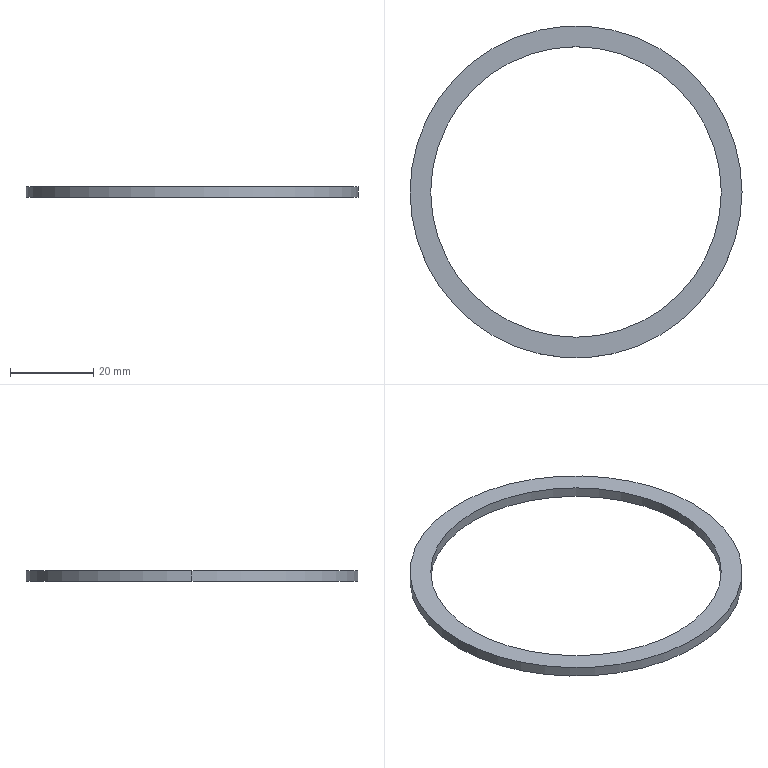Part | SolidWorks | features Extrusion 1 | 1 solid | 6 faces | box 80 x 80 x 2.5 mm | volume 2945 mm3 | cylinder 4 | plane 2 | commonest cylinder face diameters 70 x2 80 x2
STEP:
#1=CARTESIAN_POINT('',(-35.,0.,2.5));
#2=VERTEX_POINT('',#1);
#3=CARTESIAN_POINT('',(35.,0.,2.5));
#4=VERTEX_POINT('',#3);
#5=CARTESIAN_POINT('',(0.,0.,2.5));
#6=DIRECTION('',(0.,0.,1.));
#7=DIRECTION('',(1.,0.,0.));
#8=AXIS2_PLACEMENT_3D('',#5,#6,#7);
#9=CIRCLE('',#8,35.);
#10=EDGE_CURVE('',#2,#4,#9,.T.);
#11=ORIENTED_EDGE('',*,*,#10,.T.);
#12=CARTESIAN_POINT('',(35.,0.,0.));
#13=VERTEX_POINT('',#12);
#14=CARTESIAN_POINT('',(35.,0.,2.5));
#15=DIRECTION('',(0.,0.,-1.));
#16=VECTOR('',#15,1000.);
#17=LINE('',#14,#16);
#18=EDGE_CURVE('',#4,#13,#17,.T.);
#19=ORIENTED_EDGE('',*,*,#18,.T.);
#20=CARTESIAN_POINT('',(-35.,0.,0.));
#21=VERTEX_POINT('',#20);
#22=CARTESIAN_POINT('',(0.,0.,0.));
#23=DIRECTION('',(0.,0.,1.));
#24=DIRECTION('',(1.,0.,0.));
#25=AXIS2_PLACEMENT_3D('',#22,#23,#24);
#26=CIRCLE('',#25,35.);
#27=EDGE_CURVE('',#21,#13,#26,.T.);
#28=ORIENTED_EDGE('',*,*,#27,.F.);
#29=CARTESIAN_POINT('',(-35.,0.,2.5));
#30=DIRECTION('',(0.,0.,-1.));
#31=VECTOR('',#30,1000.);
#32=LINE('',#29,#31);
#33=EDGE_CURVE('',#2,#21,#32,.T.);
#34=ORIENTED_EDGE('',*,*,#33,.F.);
#35=EDGE_LOOP('',(#11,#19,#28,#34));
#36=FACE_OUTER_BOUND('',#35,.T.);
#37=CARTESIAN_POINT('',(0.,0.,2.5));
#38=DIRECTION('',(0.,0.,-1.));
#39=DIRECTION('',(-1.,0.,0.));
#40=AXIS2_PLACEMENT_3D('',#37,#38,#39);
#41=CYLINDRICAL_SURFACE('',#40,35.);
#42=ADVANCED_FACE('',(#36),#41,.F.);
#43=CARTESIAN_POINT('',(40.,0.,2.5));
#44=VERTEX_POINT('',#43);
#45=CARTESIAN_POINT('',(-40.,0.,2.5));
#46=VERTEX_POINT('',#45);
#47=CARTESIAN_POINT('',(0.,0.,2.5));
#48=DIRECTION('',(0.,0.,1.));
#49=DIRECTION('',(1.,0.,0.));
#50=AXIS2_PLACEMENT_3D('',#47,#48,#49);
#51=CIRCLE('',#50,40.);
#52=EDGE_CURVE('',#44,#46,#51,.T.);
#53=ORIENTED_EDGE('',*,*,#52,.F.);
#54=CARTESIAN_POINT('',(40.,0.,0.));
#55=VERTEX_POINT('',#54);
#56=CARTESIAN_POINT('',(40.,0.,2.5));
#57=DIRECTION('',(0.,0.,-1.));
#58=VECTOR('',#57,1000.);
#59=LINE('',#56,#58);
#60=EDGE_CURVE('',#44,#55,#59,.T.);
#61=ORIENTED_EDGE('',*,*,#60,.T.);
#62=CARTESIAN_POINT('',(-40.,0.,0.));
#63=VERTEX_POINT('',#62);
#64=CARTESIAN_POINT('',(0.,0.,0.));
#65=DIRECTION('',(0.,0.,1.));
#66=DIRECTION('',(1.,0.,0.));
#67=AXIS2_PLACEMENT_3D('',#64,#65,#66);
#68=CIRCLE('',#67,40.);
#69=EDGE_CURVE('',#55,#63,#68,.T.);
#70=ORIENTED_EDGE('',*,*,#69,.T.);
#71=CARTESIAN_POINT('',(-40.,0.,2.5));
#72=DIRECTION('',(0.,0.,-1.));
#73=VECTOR('',#72,1000.);
#74=LINE('',#71,#73);
#75=EDGE_CURVE('',#46,#63,#74,.T.);
#76=ORIENTED_EDGE('',*,*,#75,.F.);
#77=EDGE_LOOP('',(#53,#61,#70,#76));
#78=FACE_OUTER_BOUND('',#77,.T.);
#79=CARTESIAN_POINT('',(0.,0.,2.5));
#80=DIRECTION('',(0.,0.,-1.));
#81=DIRECTION('',(-1.,0.,0.));
#82=AXIS2_PLACEMENT_3D('',#79,#80,#81);
#83=CYLINDRICAL_SURFACE('',#82,40.);
#84=ADVANCED_FACE('',(#78),#83,.T.);
#85=CARTESIAN_POINT('',(0.,0.,2.5));
#86=DIRECTION('',(0.,0.,1.));
#87=DIRECTION('',(1.,0.,0.));
#88=AXIS2_PLACEMENT_3D('',#85,#86,#87);
#89=CIRCLE('',#88,40.);
#90=EDGE_CURVE('',#46,#44,#89,.T.);
#91=ORIENTED_EDGE('',*,*,#90,.T.);
#92=ORIENTED_EDGE('',*,*,#52,.T.);
#93=EDGE_LOOP('',(#91,#92));
#94=FACE_OUTER_BOUND('',#93,.T.);
#95=ORIENTED_EDGE('',*,*,#10,.F.);
#96=CARTESIAN_POINT('',(0.,0.,2.5));
#97=DIRECTION('',(0.,0.,1.));
#98=DIRECTION('',(1.,0.,0.));
#99=AXIS2_PLACEMENT_3D('',#96,#97,#98);
#100=CIRCLE('',#99,35.);
#101=EDGE_CURVE('',#4,#2,#100,.T.);
#102=ORIENTED_EDGE('',*,*,#101,.F.);
#103=EDGE_LOOP('',(#95,#102));
#104=FACE_BOUND('',#103,.T.);
#105=CARTESIAN_POINT('',(0.,0.,2.5));
#106=DIRECTION('',(0.,0.,1.));
#107=DIRECTION('',(1.,0.,0.));
#108=AXIS2_PLACEMENT_3D('',#105,#106,#107);
#109=PLANE('',#108);
#110=ADVANCED_FACE('',(#94,#104),#109,.T.);
#111=CARTESIAN_POINT('',(0.,0.,0.));
#112=DIRECTION('',(0.,0.,1.));
#113=DIRECTION('',(1.,0.,0.));
#114=AXIS2_PLACEMENT_3D('',#111,#112,#113);
#115=CIRCLE('',#114,40.);
#116=EDGE_CURVE('',#63,#55,#115,.T.);
#117=ORIENTED_EDGE('',*,*,#116,.F.);
#118=ORIENTED_EDGE('',*,*,#69,.F.);
#119=EDGE_LOOP('',(#117,#118));
#120=FACE_OUTER_BOUND('',#119,.T.);
#121=ORIENTED_EDGE('',*,*,#27,.T.);
#122=CARTESIAN_POINT('',(0.,0.,0.));
#123=DIRECTION('',(0.,0.,1.));
#124=DIRECTION('',(1.,0.,0.));
#125=AXIS2_PLACEMENT_3D('',#122,#123,#124);
#126=CIRCLE('',#125,35.);
#127=EDGE_CURVE('',#13,#21,#126,.T.);
#128=ORIENTED_EDGE('',*,*,#127,.T.);
#129=EDGE_LOOP('',(#121,#128));
#130=FACE_BOUND('',#129,.T.);
#131=CARTESIAN_POINT('',(0.,0.,0.));
#132=DIRECTION('',(0.,0.,1.));
#133=DIRECTION('',(1.,0.,0.));
#134=AXIS2_PLACEMENT_3D('',#131,#132,#133);
#135=PLANE('',#134);
#136=ADVANCED_FACE('',(#120,#130),#135,.F.);
#137=ORIENTED_EDGE('',*,*,#60,.F.);
#138=ORIENTED_EDGE('',*,*,#90,.F.);
#139=ORIENTED_EDGE('',*,*,#75,.T.);
#140=ORIENTED_EDGE('',*,*,#116,.T.);
#141=EDGE_LOOP('',(#137,#138,#139,#140));
#142=FACE_OUTER_BOUND('',#141,.T.);
#143=CARTESIAN_POINT('',(0.,0.,2.5));
#144=DIRECTION('',(0.,0.,-1.));
#145=DIRECTION('',(-1.,0.,0.));
#146=AXIS2_PLACEMENT_3D('',#143,#144,#145);
#147=CYLINDRICAL_SURFACE('',#146,40.);
#148=ADVANCED_FACE('',(#142),#147,.T.);
#149=ORIENTED_EDGE('',*,*,#18,.F.);
#150=ORIENTED_EDGE('',*,*,#101,.T.);
#151=ORIENTED_EDGE('',*,*,#33,.T.);
#152=ORIENTED_EDGE('',*,*,#127,.F.);
#153=EDGE_LOOP('',(#149,#150,#151,#152));
#154=FACE_OUTER_BOUND('',#153,.T.);
#155=CARTESIAN_POINT('',(0.,0.,2.5));
#156=DIRECTION('',(0.,0.,-1.));
#157=DIRECTION('',(-1.,0.,0.));
#158=AXIS2_PLACEMENT_3D('',#155,#156,#157);
#159=CYLINDRICAL_SURFACE('',#158,35.);
#160=ADVANCED_FACE('',(#154),#159,.F.);
#161=CLOSED_SHELL('',(#42,#84,#110,#136,#148,#160));
#162=MANIFOLD_SOLID_BREP('',#161);
#163=CARTESIAN_POINT('',(0.,0.,0.));
#164=DIRECTION('',(0.,0.,1.));
#165=DIRECTION('',(1.,0.,0.));
#166=AXIS2_PLACEMENT_3D('',#163,#164,#165);
#167=(LENGTH_UNIT()NAMED_UNIT(*)SI_UNIT(.MILLI.,.METRE.));
#168=UNCERTAINTY_MEASURE_WITH_UNIT(LENGTH_MEASURE(0.00001),#167,'','');
#169=(NAMED_UNIT(*)PLANE_ANGLE_UNIT()SI_UNIT($,.RADIAN.));
#170=(NAMED_UNIT(*)SI_UNIT($,.STERADIAN.)SOLID_ANGLE_UNIT());
#171=(GEOMETRIC_REPRESENTATION_CONTEXT(3)GLOBAL_UNCERTAINTY_ASSIGNED_CONTEXT((#168))GLOBAL_UNIT_ASSIGNED_CONTEXT((#167,#169,#170))REPRESENTATION_CONTEXT('',''));
#172=ADVANCED_BREP_SHAPE_REPRESENTATION('',(#162,#166),#171);